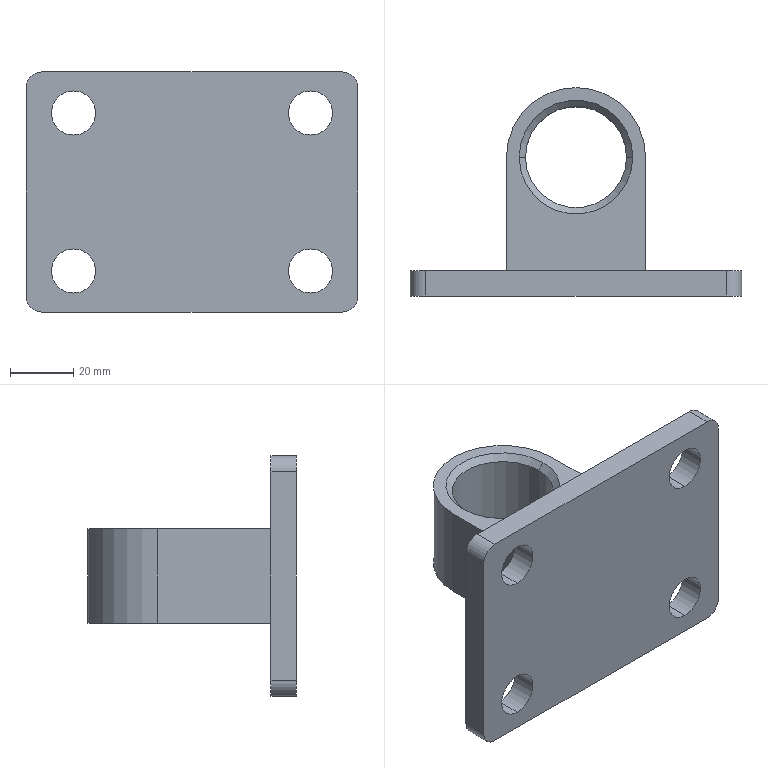Part | SolidWorks | features MirrorStock 1 | 2 solids | 30 faces | box 105 x 66 x 76 mm | volume 104524 mm3 | cylinder 15 | plane 11 | cone 4 | commonest cylinder face diameters 14 x8 10 x4 32 x2 44 x1
STEP:
#1=CARTESIAN_POINT('',(37.5,8.,18.));
#2=VERTEX_POINT('',#1);
#3=CARTESIAN_POINT('',(37.5,8.,32.));
#4=VERTEX_POINT('',#3);
#5=CARTESIAN_POINT('',(37.5,8.,25.));
#6=DIRECTION('',(0.,-1.,0.));
#7=DIRECTION('',(0.,0.,-1.));
#8=AXIS2_PLACEMENT_3D('',#5,#6,#7);
#9=CIRCLE('',#8,7.);
#10=EDGE_CURVE('',#2,#4,#9,.T.);
#11=ORIENTED_EDGE('',*,*,#10,.F.);
#12=CARTESIAN_POINT('',(37.5,0.,18.));
#13=VERTEX_POINT('',#12);
#14=CARTESIAN_POINT('',(37.5,8.,18.));
#15=DIRECTION('',(0.,-1.,0.));
#16=VECTOR('',#15,1000.);
#17=LINE('',#14,#16);
#18=EDGE_CURVE('',#2,#13,#17,.T.);
#19=ORIENTED_EDGE('',*,*,#18,.T.);
#20=CARTESIAN_POINT('',(37.5,0.,32.));
#21=VERTEX_POINT('',#20);
#22=CARTESIAN_POINT('',(37.5,0.,25.));
#23=DIRECTION('',(0.,-1.,0.));
#24=DIRECTION('',(0.,0.,-1.));
#25=AXIS2_PLACEMENT_3D('',#22,#23,#24);
#26=CIRCLE('',#25,7.);
#27=EDGE_CURVE('',#13,#21,#26,.T.);
#28=ORIENTED_EDGE('',*,*,#27,.T.);
#29=CARTESIAN_POINT('',(37.5,8.,32.));
#30=DIRECTION('',(0.,-1.,0.));
#31=VECTOR('',#30,1000.);
#32=LINE('',#29,#31);
#33=EDGE_CURVE('',#4,#21,#32,.T.);
#34=ORIENTED_EDGE('',*,*,#33,.F.);
#35=EDGE_LOOP('',(#11,#19,#28,#34));
#36=FACE_OUTER_BOUND('',#35,.T.);
#37=CARTESIAN_POINT('',(37.5,8.,25.));
#38=DIRECTION('',(0.,-1.,0.));
#39=DIRECTION('',(0.,0.,1.));
#40=AXIS2_PLACEMENT_3D('',#37,#38,#39);
#41=CYLINDRICAL_SURFACE('',#40,7.);
#42=ADVANCED_FACE('',(#36),#41,.F.);
#43=CARTESIAN_POINT('',(-37.5,8.,18.));
#44=VERTEX_POINT('',#43);
#45=CARTESIAN_POINT('',(-37.5,8.,32.));
#46=VERTEX_POINT('',#45);
#47=CARTESIAN_POINT('',(-37.5,8.,25.));
#48=DIRECTION('',(0.,-1.,0.));
#49=DIRECTION('',(0.,0.,1.));
#50=AXIS2_PLACEMENT_3D('',#47,#48,#49);
#51=CIRCLE('',#50,7.);
#52=EDGE_CURVE('',#44,#46,#51,.T.);
#53=ORIENTED_EDGE('',*,*,#52,.F.);
#54=CARTESIAN_POINT('',(-37.5,0.,18.));
#55=VERTEX_POINT('',#54);
#56=CARTESIAN_POINT('',(-37.5,8.,18.));
#57=DIRECTION('',(0.,-1.,0.));
#58=VECTOR('',#57,1000.);
#59=LINE('',#56,#58);
#60=EDGE_CURVE('',#44,#55,#59,.T.);
#61=ORIENTED_EDGE('',*,*,#60,.T.);
#62=CARTESIAN_POINT('',(-37.5,0.,32.));
#63=VERTEX_POINT('',#62);
#64=CARTESIAN_POINT('',(-37.5,0.,25.));
#65=DIRECTION('',(0.,-1.,0.));
#66=DIRECTION('',(0.,0.,1.));
#67=AXIS2_PLACEMENT_3D('',#64,#65,#66);
#68=CIRCLE('',#67,7.);
#69=EDGE_CURVE('',#55,#63,#68,.T.);
#70=ORIENTED_EDGE('',*,*,#69,.T.);
#71=CARTESIAN_POINT('',(-37.5,8.,32.));
#72=DIRECTION('',(0.,-1.,0.));
#73=VECTOR('',#72,1000.);
#74=LINE('',#71,#73);
#75=EDGE_CURVE('',#46,#63,#74,.T.);
#76=ORIENTED_EDGE('',*,*,#75,.F.);
#77=EDGE_LOOP('',(#53,#61,#70,#76));
#78=FACE_OUTER_BOUND('',#77,.T.);
#79=CARTESIAN_POINT('',(-37.5,8.,25.));
#80=DIRECTION('',(0.,-1.,0.));
#81=DIRECTION('',(0.,0.,1.));
#82=AXIS2_PLACEMENT_3D('',#79,#80,#81);
#83=CYLINDRICAL_SURFACE('',#82,7.);
#84=ADVANCED_FACE('',(#78),#83,.F.);
#85=CARTESIAN_POINT('',(37.5,8.,-32.));
#86=VERTEX_POINT('',#85);
#87=CARTESIAN_POINT('',(37.5,8.,-18.));
#88=VERTEX_POINT('',#87);
#89=CARTESIAN_POINT('',(37.5,8.,-25.));
#90=DIRECTION('',(0.,-1.,0.));
#91=DIRECTION('',(0.,0.,1.));
#92=AXIS2_PLACEMENT_3D('',#89,#90,#91);
#93=CIRCLE('',#92,7.);
#94=EDGE_CURVE('',#86,#88,#93,.T.);
#95=ORIENTED_EDGE('',*,*,#94,.F.);
#96=CARTESIAN_POINT('',(37.5,0.,-32.));
#97=VERTEX_POINT('',#96);
#98=CARTESIAN_POINT('',(37.5,8.,-32.));
#99=DIRECTION('',(0.,-1.,0.));
#100=VECTOR('',#99,1000.);
#101=LINE('',#98,#100);
#102=EDGE_CURVE('',#86,#97,#101,.T.);
#103=ORIENTED_EDGE('',*,*,#102,.T.);
#104=CARTESIAN_POINT('',(37.5,0.,-18.));
#105=VERTEX_POINT('',#104);
#106=CARTESIAN_POINT('',(37.5,0.,-25.));
#107=DIRECTION('',(0.,-1.,0.));
#108=DIRECTION('',(0.,0.,1.));
#109=AXIS2_PLACEMENT_3D('',#106,#107,#108);
#110=CIRCLE('',#109,7.);
#111=EDGE_CURVE('',#97,#105,#110,.T.);
#112=ORIENTED_EDGE('',*,*,#111,.T.);
#113=CARTESIAN_POINT('',(37.5,8.,-18.));
#114=DIRECTION('',(0.,-1.,0.));
#115=VECTOR('',#114,1000.);
#116=LINE('',#113,#115);
#117=EDGE_CURVE('',#88,#105,#116,.T.);
#118=ORIENTED_EDGE('',*,*,#117,.F.);
#119=EDGE_LOOP('',(#95,#103,#112,#118));
#120=FACE_OUTER_BOUND('',#119,.T.);
#121=CARTESIAN_POINT('',(37.5,8.,-25.));
#122=DIRECTION('',(0.,-1.,0.));
#123=DIRECTION('',(0.,0.,1.));
#124=AXIS2_PLACEMENT_3D('',#121,#122,#123);
#125=CYLINDRICAL_SURFACE('',#124,7.);
#126=ADVANCED_FACE('',(#120),#125,.F.);
#127=CARTESIAN_POINT('',(-37.5,8.,-32.));
#128=VERTEX_POINT('',#127);
#129=CARTESIAN_POINT('',(-37.5,8.,-18.));
#130=VERTEX_POINT('',#129);
#131=CARTESIAN_POINT('',(-37.5,8.,-25.));
#132=DIRECTION('',(0.,-1.,0.));
#133=DIRECTION('',(0.,0.,-1.));
#134=AXIS2_PLACEMENT_3D('',#131,#132,#133);
#135=CIRCLE('',#134,7.);
#136=EDGE_CURVE('',#128,#130,#135,.T.);
#137=ORIENTED_EDGE('',*,*,#136,.F.);
#138=CARTESIAN_POINT('',(-37.5,0.,-32.));
#139=VERTEX_POINT('',#138);
#140=CARTESIAN_POINT('',(-37.5,8.,-32.));
#141=DIRECTION('',(0.,-1.,0.));
#142=VECTOR('',#141,1000.);
#143=LINE('',#140,#142);
#144=EDGE_CURVE('',#128,#139,#143,.T.);
#145=ORIENTED_EDGE('',*,*,#144,.T.);
#146=CARTESIAN_POINT('',(-37.5,0.,-18.));
#147=VERTEX_POINT('',#146);
#148=CARTESIAN_POINT('',(-37.5,0.,-25.));
#149=DIRECTION('',(0.,-1.,0.));
#150=DIRECTION('',(0.,0.,-1.));
#151=AXIS2_PLACEMENT_3D('',#148,#149,#150);
#152=CIRCLE('',#151,7.);
#153=EDGE_CURVE('',#139,#147,#152,.T.);
#154=ORIENTED_EDGE('',*,*,#153,.T.);
#155=CARTESIAN_POINT('',(-37.5,8.,-18.));
#156=DIRECTION('',(0.,-1.,0.));
#157=VECTOR('',#156,1000.);
#158=LINE('',#155,#157);
#159=EDGE_CURVE('',#130,#147,#158,.T.);
#160=ORIENTED_EDGE('',*,*,#159,.F.);
#161=EDGE_LOOP('',(#137,#145,#154,#160));
#162=FACE_OUTER_BOUND('',#161,.T.);
#163=CARTESIAN_POINT('',(-37.5,8.,-25.));
#164=DIRECTION('',(0.,-1.,0.));
#165=DIRECTION('',(0.,0.,1.));
#166=AXIS2_PLACEMENT_3D('',#163,#164,#165);
#167=CYLINDRICAL_SURFACE('',#166,7.);
#168=ADVANCED_FACE('',(#162),#167,.F.);
#169=CARTESIAN_POINT('',(-37.5,8.,25.));
#170=DIRECTION('',(0.,-1.,0.));
#171=DIRECTION('',(0.,0.,1.));
#172=AXIS2_PLACEMENT_3D('',#169,#170,#171);
#173=CIRCLE('',#172,7.);
#174=EDGE_CURVE('',#46,#44,#173,.T.);
#175=ORIENTED_EDGE('',*,*,#174,.T.);
#176=ORIENTED_EDGE('',*,*,#52,.T.);
#177=EDGE_LOOP('',(#175,#176));
#178=FACE_BOUND('',#177,.T.);
#179=CARTESIAN_POINT('',(-37.5,8.,-25.));
#180=DIRECTION('',(0.,-1.,0.));
#181=DIRECTION('',(0.,0.,-1.));
#182=AXIS2_PLACEMENT_3D('',#179,#180,#181);
#183=CIRCLE('',#182,7.);
#184=EDGE_CURVE('',#130,#128,#183,.T.);
#185=ORIENTED_EDGE('',*,*,#184,.T.);
#186=ORIENTED_EDGE('',*,*,#136,.T.);
#187=EDGE_LOOP('',(#185,#186));
#188=FACE_BOUND('',#187,.T.);
#189=CARTESIAN_POINT('',(47.5,8.,-38.));
#190=VERTEX_POINT('',#189);
#191=CARTESIAN_POINT('',(52.5,8.,-33.));
#192=VERTEX_POINT('',#191);
#193=CARTESIAN_POINT('',(47.5,8.,-33.));
#194=DIRECTION('',(0.,-1.,0.));
#195=DIRECTION('',(0.,0.,-1.));
#196=AXIS2_PLACEMENT_3D('',#193,#194,#195);
#197=CIRCLE('',#196,5.);
#198=EDGE_CURVE('',#190,#192,#197,.T.);
#199=ORIENTED_EDGE('',*,*,#198,.F.);
#200=CARTESIAN_POINT('',(-47.5,8.,-38.));
#201=VERTEX_POINT('',#200);
#202=CARTESIAN_POINT('',(-47.5,8.,-38.));
#203=DIRECTION('',(1.,0.,0.));
#204=VECTOR('',#203,1000.);
#205=LINE('',#202,#204);
#206=EDGE_CURVE('',#201,#190,#205,.T.);
#207=ORIENTED_EDGE('',*,*,#206,.F.);
#208=CARTESIAN_POINT('',(-52.5,8.,-33.));
#209=VERTEX_POINT('',#208);
#210=CARTESIAN_POINT('',(-47.5,8.,-33.));
#211=DIRECTION('',(0.,-1.,0.));
#212=DIRECTION('',(0.,0.,1.));
#213=AXIS2_PLACEMENT_3D('',#210,#211,#212);
#214=CIRCLE('',#213,5.);
#215=EDGE_CURVE('',#209,#201,#214,.T.);
#216=ORIENTED_EDGE('',*,*,#215,.F.);
#217=CARTESIAN_POINT('',(-52.5,8.,33.));
#218=VERTEX_POINT('',#217);
#219=CARTESIAN_POINT('',(-52.5,8.,-33.));
#220=DIRECTION('',(0.,0.,-1.));
#221=VECTOR('',#220,1000.);
#222=LINE('',#219,#221);
#223=EDGE_CURVE('',#218,#209,#222,.T.);
#224=ORIENTED_EDGE('',*,*,#223,.F.);
#225=CARTESIAN_POINT('',(-47.5,8.,38.));
#226=VERTEX_POINT('',#225);
#227=CARTESIAN_POINT('',(-47.5,8.,33.));
#228=DIRECTION('',(0.,-1.,0.));
#229=DIRECTION('',(0.,0.,1.));
#230=AXIS2_PLACEMENT_3D('',#227,#228,#229);
#231=CIRCLE('',#230,5.);
#232=EDGE_CURVE('',#226,#218,#231,.T.);
#233=ORIENTED_EDGE('',*,*,#232,.F.);
#234=CARTESIAN_POINT('',(47.5,8.,38.));
#235=VERTEX_POINT('',#234);
#236=CARTESIAN_POINT('',(-47.5,8.,38.));
#237=DIRECTION('',(-1.,0.,0.));
#238=VECTOR('',#237,1000.);
#239=LINE('',#236,#238);
#240=EDGE_CURVE('',#235,#226,#239,.T.);
#241=ORIENTED_EDGE('',*,*,#240,.F.);
#242=CARTESIAN_POINT('',(52.5,8.,33.));
#243=VERTEX_POINT('',#242);
#244=CARTESIAN_POINT('',(47.5,8.,33.));
#245=DIRECTION('',(0.,-1.,0.));
#246=DIRECTION('',(0.,0.,1.));
#247=AXIS2_PLACEMENT_3D('',#244,#245,#246);
#248=CIRCLE('',#247,5.);
#249=EDGE_CURVE('',#243,#235,#248,.T.);
#250=ORIENTED_EDGE('',*,*,#249,.F.);
#251=CARTESIAN_POINT('',(52.5,8.,-33.));
#252=DIRECTION('',(0.,0.,1.));
#253=VECTOR('',#252,1000.);
#254=LINE('',#251,#253);
#255=EDGE_CURVE('',#192,#243,#254,.T.);
#256=ORIENTED_EDGE('',*,*,#255,.F.);
#257=EDGE_LOOP('',(#199,#207,#216,#224,#233,#241,#250,#256));
#258=FACE_OUTER_BOUND('',#257,.T.);
#259=CARTESIAN_POINT('',(37.5,8.,-25.));
#260=DIRECTION('',(0.,-1.,0.));
#261=DIRECTION('',(0.,0.,1.));
#262=AXIS2_PLACEMENT_3D('',#259,#260,#261);
#263=CIRCLE('',#262,7.);
#264=EDGE_CURVE('',#88,#86,#263,.T.);
#265=ORIENTED_EDGE('',*,*,#264,.T.);
#266=ORIENTED_EDGE('',*,*,#94,.T.);
#267=EDGE_LOOP('',(#265,#266));
#268=FACE_BOUND('',#267,.T.);
#269=CARTESIAN_POINT('',(37.5,8.,25.));
#270=DIRECTION('',(0.,-1.,0.));
#271=DIRECTION('',(0.,0.,-1.));
#272=AXIS2_PLACEMENT_3D('',#269,#270,#271);
#273=CIRCLE('',#272,7.);
#274=EDGE_CURVE('',#4,#2,#273,.T.);
#275=ORIENTED_EDGE('',*,*,#274,.T.);
#276=ORIENTED_EDGE('',*,*,#10,.T.);
#277=EDGE_LOOP('',(#275,#276));
#278=FACE_BOUND('',#277,.T.);
#279=CARTESIAN_POINT('',(47.5,8.,-33.));
#280=DIRECTION('',(0.,1.,0.));
#281=DIRECTION('',(0.,0.,-1.));
#282=AXIS2_PLACEMENT_3D('',#279,#280,#281);
#283=PLANE('',#282);
#284=ADVANCED_FACE('',(#178,#188,#258,#268,#278),#283,.T.);
#285=CARTESIAN_POINT('',(47.5,0.,-38.));
#286=VERTEX_POINT('',#285);
#287=CARTESIAN_POINT('',(52.5,0.,-33.));
#288=VERTEX_POINT('',#287);
#289=CARTESIAN_POINT('',(47.5,0.,-33.));
#290=DIRECTION('',(0.,-1.,0.));
#291=DIRECTION('',(0.,0.,-1.));
#292=AXIS2_PLACEMENT_3D('',#289,#290,#291);
#293=CIRCLE('',#292,5.);
#294=EDGE_CURVE('',#286,#288,#293,.T.);
#295=ORIENTED_EDGE('',*,*,#294,.T.);
#296=CARTESIAN_POINT('',(52.5,0.,33.));
#297=VERTEX_POINT('',#296);
#298=CARTESIAN_POINT('',(52.5,0.,-33.));
#299=DIRECTION('',(0.,0.,1.));
#300=VECTOR('',#299,1000.);
#301=LINE('',#298,#300);
#302=EDGE_CURVE('',#288,#297,#301,.T.);
#303=ORIENTED_EDGE('',*,*,#302,.T.);
#304=CARTESIAN_POINT('',(47.5,0.,38.));
#305=VERTEX_POINT('',#304);
#306=CARTESIAN_POINT('',(47.5,0.,33.));
#307=DIRECTION('',(0.,-1.,0.));
#308=DIRECTION('',(0.,0.,1.));
#309=AXIS2_PLACEMENT_3D('',#306,#307,#308);
#310=CIRCLE('',#309,5.);
#311=EDGE_CURVE('',#297,#305,#310,.T.);
#312=ORIENTED_EDGE('',*,*,#311,.T.);
#313=CARTESIAN_POINT('',(-47.5,0.,38.));
#314=VERTEX_POINT('',#313);
#315=CARTESIAN_POINT('',(-47.5,0.,38.));
#316=DIRECTION('',(-1.,0.,0.));
#317=VECTOR('',#316,1000.);
#318=LINE('',#315,#317);
#319=EDGE_CURVE('',#305,#314,#318,.T.);
#320=ORIENTED_EDGE('',*,*,#319,.T.);
#321=CARTESIAN_POINT('',(-52.5,0.,33.));
#322=VERTEX_POINT('',#321);
#323=CARTESIAN_POINT('',(-47.5,0.,33.));
#324=DIRECTION('',(0.,-1.,0.));
#325=DIRECTION('',(0.,0.,1.));
#326=AXIS2_PLACEMENT_3D('',#323,#324,#325);
#327=CIRCLE('',#326,5.);
#328=EDGE_CURVE('',#314,#322,#327,.T.);
#329=ORIENTED_EDGE('',*,*,#328,.T.);
#330=CARTESIAN_POINT('',(-52.5,0.,-33.));
#331=VERTEX_POINT('',#330);
#332=CARTESIAN_POINT('',(-52.5,0.,-33.));
#333=DIRECTION('',(0.,0.,-1.));
#334=VECTOR('',#333,1000.);
#335=LINE('',#332,#334);
#336=EDGE_CURVE('',#322,#331,#335,.T.);
#337=ORIENTED_EDGE('',*,*,#336,.T.);
#338=CARTESIAN_POINT('',(-47.5,0.,-38.));
#339=VERTEX_POINT('',#338);
#340=CARTESIAN_POINT('',(-47.5,0.,-33.));
#341=DIRECTION('',(0.,-1.,0.));
#342=DIRECTION('',(0.,0.,1.));
#343=AXIS2_PLACEMENT_3D('',#340,#341,#342);
#344=CIRCLE('',#343,5.);
#345=EDGE_CURVE('',#331,#339,#344,.T.);
#346=ORIENTED_EDGE('',*,*,#345,.T.);
#347=CARTESIAN_POINT('',(-47.5,0.,-38.));
#348=DIRECTION('',(1.,0.,0.));
#349=VECTOR('',#348,1000.);
#350=LINE('',#347,#349);
#351=EDGE_CURVE('',#339,#286,#350,.T.);
#352=ORIENTED_EDGE('',*,*,#351,.T.);
#353=EDGE_LOOP('',(#295,#303,#312,#320,#329,#337,#346,#352));
#354=FACE_OUTER_BOUND('',#353,.T.);
#355=CARTESIAN_POINT('',(-37.5,0.,-25.));
#356=DIRECTION('',(0.,-1.,0.));
#357=DIRECTION('',(0.,0.,-1.));
#358=AXIS2_PLACEMENT_3D('',#355,#356,#357);
#359=CIRCLE('',#358,7.);
#360=EDGE_CURVE('',#147,#139,#359,.T.);
#361=ORIENTED_EDGE('',*,*,#360,.F.);
#362=ORIENTED_EDGE('',*,*,#153,.F.);
#363=EDGE_LOOP('',(#361,#362));
#364=FACE_BOUND('',#363,.T.);
#365=CARTESIAN_POINT('',(37.5,0.,-25.));
#366=DIRECTION('',(0.,-1.,0.));
#367=DIRECTION('',(0.,0.,1.));
#368=AXIS2_PLACEMENT_3D('',#365,#366,#367);
#369=CIRCLE('',#368,7.);
#370=EDGE_CURVE('',#105,#97,#369,.T.);
#371=ORIENTED_EDGE('',*,*,#370,.F.);
#372=ORIENTED_EDGE('',*,*,#111,.F.);
#373=EDGE_LOOP('',(#371,#372));
#374=FACE_BOUND('',#373,.T.);
#375=CARTESIAN_POINT('',(-37.5,0.,25.));
#376=DIRECTION('',(0.,-1.,0.));
#377=DIRECTION('',(0.,0.,1.));
#378=AXIS2_PLACEMENT_3D('',#375,#376,#377);
#379=CIRCLE('',#378,7.);
#380=EDGE_CURVE('',#63,#55,#379,.T.);
#381=ORIENTED_EDGE('',*,*,#380,.F.);
#382=ORIENTED_EDGE('',*,*,#69,.F.);
#383=EDGE_LOOP('',(#381,#382));
#384=FACE_BOUND('',#383,.T.);
#385=CARTESIAN_POINT('',(37.5,0.,25.));
#386=DIRECTION('',(0.,-1.,0.));
#387=DIRECTION('',(0.,0.,-1.));
#388=AXIS2_PLACEMENT_3D('',#385,#386,#387);
#389=CIRCLE('',#388,7.);
#390=EDGE_CURVE('',#21,#13,#389,.T.);
#391=ORIENTED_EDGE('',*,*,#390,.F.);
#392=ORIENTED_EDGE('',*,*,#27,.F.);
#393=EDGE_LOOP('',(#391,#392));
#394=FACE_BOUND('',#393,.T.);
#395=CARTESIAN_POINT('',(47.5,0.,-33.));
#396=DIRECTION('',(0.,1.,0.));
#397=DIRECTION('',(0.,0.,-1.));
#398=AXIS2_PLACEMENT_3D('',#395,#396,#397);
#399=PLANE('',#398);
#400=ADVANCED_FACE('',(#354,#364,#374,#384,#394),#399,.F.);
#401=ORIENTED_EDGE('',*,*,#294,.F.);
#402=CARTESIAN_POINT('',(47.5,8.,-38.));
#403=DIRECTION('',(0.,-1.,0.));
#404=VECTOR('',#403,1000.);
#405=LINE('',#402,#404);
#406=EDGE_CURVE('',#190,#286,#405,.T.);
#407=ORIENTED_EDGE('',*,*,#406,.F.);
#408=ORIENTED_EDGE('',*,*,#198,.T.);
#409=CARTESIAN_POINT('',(52.5,8.,-33.));
#410=DIRECTION('',(0.,-1.,0.));
#411=VECTOR('',#410,1000.);
#412=LINE('',#409,#411);
#413=EDGE_CURVE('',#192,#288,#412,.T.);
#414=ORIENTED_EDGE('',*,*,#413,.T.);
#415=EDGE_LOOP('',(#401,#407,#408,#414));
#416=FACE_OUTER_BOUND('',#415,.T.);
#417=CARTESIAN_POINT('',(47.5,8.,-33.));
#418=DIRECTION('',(0.,-1.,0.));
#419=DIRECTION('',(0.,0.,1.));
#420=AXIS2_PLACEMENT_3D('',#417,#418,#419);
#421=CYLINDRICAL_SURFACE('',#420,5.);
#422=ADVANCED_FACE('',(#416),#421,.T.);
#423=ORIENTED_EDGE('',*,*,#302,.F.);
#424=ORIENTED_EDGE('',*,*,#413,.F.);
#425=ORIENTED_EDGE('',*,*,#255,.T.);
#426=CARTESIAN_POINT('',(52.5,8.,33.));
#427=DIRECTION('',(0.,-1.,0.));
#428=VECTOR('',#427,1000.);
#429=LINE('',#426,#428);
#430=EDGE_CURVE('',#243,#297,#429,.T.);
#431=ORIENTED_EDGE('',*,*,#430,.T.);
#432=EDGE_LOOP('',(#423,#424,#425,#431));
#433=FACE_OUTER_BOUND('',#432,.T.);
#434=CARTESIAN_POINT('',(52.5,8.,-33.));
#435=DIRECTION('',(-1.,0.,0.));
#436=DIRECTION('',(0.,0.,-1.));
#437=AXIS2_PLACEMENT_3D('',#434,#435,#436);
#438=PLANE('',#437);
#439=ADVANCED_FACE('',(#433),#438,.F.);
#440=ORIENTED_EDGE('',*,*,#311,.F.);
#441=ORIENTED_EDGE('',*,*,#430,.F.);
#442=ORIENTED_EDGE('',*,*,#249,.T.);
#443=CARTESIAN_POINT('',(47.5,8.,38.));
#444=DIRECTION('',(0.,-1.,0.));
#445=VECTOR('',#444,1000.);
#446=LINE('',#443,#445);
#447=EDGE_CURVE('',#235,#305,#446,.T.);
#448=ORIENTED_EDGE('',*,*,#447,.T.);
#449=EDGE_LOOP('',(#440,#441,#442,#448));
#450=FACE_OUTER_BOUND('',#449,.T.);
#451=CARTESIAN_POINT('',(47.5,8.,33.));
#452=DIRECTION('',(0.,-1.,0.));
#453=DIRECTION('',(0.,0.,1.));
#454=AXIS2_PLACEMENT_3D('',#451,#452,#453);
#455=CYLINDRICAL_SURFACE('',#454,5.);
#456=ADVANCED_FACE('',(#450),#455,.T.);
#457=ORIENTED_EDGE('',*,*,#319,.F.);
#458=ORIENTED_EDGE('',*,*,#447,.F.);
#459=ORIENTED_EDGE('',*,*,#240,.T.);
#460=CARTESIAN_POINT('',(-47.5,8.,38.));
#461=DIRECTION('',(0.,-1.,0.));
#462=VECTOR('',#461,1000.);
#463=LINE('',#460,#462);
#464=EDGE_CURVE('',#226,#314,#463,.T.);
#465=ORIENTED_EDGE('',*,*,#464,.T.);
#466=EDGE_LOOP('',(#457,#458,#459,#465));
#467=FACE_OUTER_BOUND('',#466,.T.);
#468=CARTESIAN_POINT('',(-47.5,8.,38.));
#469=DIRECTION('',(0.,0.,-1.));
#470=DIRECTION('',(1.,0.,0.));
#471=AXIS2_PLACEMENT_3D('',#468,#469,#470);
#472=PLANE('',#471);
#473=ADVANCED_FACE('',(#467),#472,.F.);
#474=ORIENTED_EDGE('',*,*,#328,.F.);
#475=ORIENTED_EDGE('',*,*,#464,.F.);
#476=ORIENTED_EDGE('',*,*,#232,.T.);
#477=CARTESIAN_POINT('',(-52.5,8.,33.));
#478=DIRECTION('',(0.,-1.,0.));
#479=VECTOR('',#478,1000.);
#480=LINE('',#477,#479);
#481=EDGE_CURVE('',#218,#322,#480,.T.);
#482=ORIENTED_EDGE('',*,*,#481,.T.);
#483=EDGE_LOOP('',(#474,#475,#476,#482));
#484=FACE_OUTER_BOUND('',#483,.T.);
#485=CARTESIAN_POINT('',(-47.5,8.,33.));
#486=DIRECTION('',(0.,-1.,0.));
#487=DIRECTION('',(0.,0.,1.));
#488=AXIS2_PLACEMENT_3D('',#485,#486,#487);
#489=CYLINDRICAL_SURFACE('',#488,5.);
#490=ADVANCED_FACE('',(#484),#489,.T.);
#491=ORIENTED_EDGE('',*,*,#336,.F.);
#492=ORIENTED_EDGE('',*,*,#481,.F.);
#493=ORIENTED_EDGE('',*,*,#223,.T.);
#494=CARTESIAN_POINT('',(-52.5,8.,-33.));
#495=DIRECTION('',(0.,-1.,0.));
#496=VECTOR('',#495,1000.);
#497=LINE('',#494,#496);
#498=EDGE_CURVE('',#209,#331,#497,.T.);
#499=ORIENTED_EDGE('',*,*,#498,.T.);
#500=EDGE_LOOP('',(#491,#492,#493,#499));
#501=FACE_OUTER_BOUND('',#500,.T.);
#502=CARTESIAN_POINT('',(-52.5,8.,-33.));
#503=DIRECTION('',(1.,0.,0.));
#504=DIRECTION('',(0.,0.,1.));
#505=AXIS2_PLACEMENT_3D('',#502,#503,#504);
#506=PLANE('',#505);
#507=ADVANCED_FACE('',(#501),#506,.F.);
#508=ORIENTED_EDGE('',*,*,#345,.F.);
#509=ORIENTED_EDGE('',*,*,#498,.F.);
#510=ORIENTED_EDGE('',*,*,#215,.T.);
#511=CARTESIAN_POINT('',(-47.5,8.,-38.));
#512=DIRECTION('',(0.,-1.,0.));
#513=VECTOR('',#512,1000.);
#514=LINE('',#511,#513);
#515=EDGE_CURVE('',#201,#339,#514,.T.);
#516=ORIENTED_EDGE('',*,*,#515,.T.);
#517=EDGE_LOOP('',(#508,#509,#510,#516));
#518=FACE_OUTER_BOUND('',#517,.T.);
#519=CARTESIAN_POINT('',(-47.5,8.,-33.));
#520=DIRECTION('',(0.,-1.,0.));
#521=DIRECTION('',(0.,0.,1.));
#522=AXIS2_PLACEMENT_3D('',#519,#520,#521);
#523=CYLINDRICAL_SURFACE('',#522,5.);
#524=ADVANCED_FACE('',(#518),#523,.T.);
#525=ORIENTED_EDGE('',*,*,#351,.F.);
#526=ORIENTED_EDGE('',*,*,#515,.F.);
#527=ORIENTED_EDGE('',*,*,#206,.T.);
#528=ORIENTED_EDGE('',*,*,#406,.T.);
#529=EDGE_LOOP('',(#525,#526,#527,#528));
#530=FACE_OUTER_BOUND('',#529,.T.);
#531=CARTESIAN_POINT('',(-47.5,8.,-38.));
#532=DIRECTION('',(0.,0.,1.));
#533=DIRECTION('',(-1.,0.,0.));
#534=AXIS2_PLACEMENT_3D('',#531,#532,#533);
#535=PLANE('',#534);
#536=ADVANCED_FACE('',(#530),#535,.F.);
#537=ORIENTED_EDGE('',*,*,#144,.F.);
#538=ORIENTED_EDGE('',*,*,#184,.F.);
#539=ORIENTED_EDGE('',*,*,#159,.T.);
#540=ORIENTED_EDGE('',*,*,#360,.T.);
#541=EDGE_LOOP('',(#537,#538,#539,#540));
#542=FACE_OUTER_BOUND('',#541,.T.);
#543=CARTESIAN_POINT('',(-37.5,8.,-25.));
#544=DIRECTION('',(0.,-1.,0.));
#545=DIRECTION('',(0.,0.,1.));
#546=AXIS2_PLACEMENT_3D('',#543,#544,#545);
#547=CYLINDRICAL_SURFACE('',#546,7.);
#548=ADVANCED_FACE('',(#542),#547,.F.);
#549=ORIENTED_EDGE('',*,*,#102,.F.);
#550=ORIENTED_EDGE('',*,*,#264,.F.);
#551=ORIENTED_EDGE('',*,*,#117,.T.);
#552=ORIENTED_EDGE('',*,*,#370,.T.);
#553=EDGE_LOOP('',(#549,#550,#551,#552));
#554=FACE_OUTER_BOUND('',#553,.T.);
#555=CARTESIAN_POINT('',(37.5,8.,-25.));
#556=DIRECTION('',(0.,-1.,0.));
#557=DIRECTION('',(0.,0.,1.));
#558=AXIS2_PLACEMENT_3D('',#555,#556,#557);
#559=CYLINDRICAL_SURFACE('',#558,7.);
#560=ADVANCED_FACE('',(#554),#559,.F.);
#561=ORIENTED_EDGE('',*,*,#60,.F.);
#562=ORIENTED_EDGE('',*,*,#174,.F.);
#563=ORIENTED_EDGE('',*,*,#75,.T.);
#564=ORIENTED_EDGE('',*,*,#380,.T.);
#565=EDGE_LOOP('',(#561,#562,#563,#564));
#566=FACE_OUTER_BOUND('',#565,.T.);
#567=CARTESIAN_POINT('',(-37.5,8.,25.));
#568=DIRECTION('',(0.,-1.,0.));
#569=DIRECTION('',(0.,0.,1.));
#570=AXIS2_PLACEMENT_3D('',#567,#568,#569);
#571=CYLINDRICAL_SURFACE('',#570,7.);
#572=ADVANCED_FACE('',(#566),#571,.F.);
#573=ORIENTED_EDGE('',*,*,#18,.F.);
#574=ORIENTED_EDGE('',*,*,#274,.F.);
#575=ORIENTED_EDGE('',*,*,#33,.T.);
#576=ORIENTED_EDGE('',*,*,#390,.T.);
#577=EDGE_LOOP('',(#573,#574,#575,#576));
#578=FACE_OUTER_BOUND('',#577,.T.);
#579=CARTESIAN_POINT('',(37.5,8.,25.));
#580=DIRECTION('',(0.,-1.,0.));
#581=DIRECTION('',(0.,0.,1.));
#582=AXIS2_PLACEMENT_3D('',#579,#580,#581);
#583=CYLINDRICAL_SURFACE('',#582,7.);
#584=ADVANCED_FACE('',(#578),#583,.F.);
#585=CLOSED_SHELL('',(#42,#84,#126,#168,#284,#400,#422,#439,#456,#473,#490,#507,#524,#536,#548,#560,#572,#584));
#586=MANIFOLD_SOLID_BREP('',#585);
#587=CARTESIAN_POINT('',(-16.,44.,13.));
#588=VERTEX_POINT('',#587);
#589=CARTESIAN_POINT('',(16.,44.,13.));
#590=VERTEX_POINT('',#589);
#591=CARTESIAN_POINT('',(0.,44.,13.));
#592=DIRECTION('',(0.,0.,-1.));
#593=DIRECTION('',(1.,0.,0.));
#594=AXIS2_PLACEMENT_3D('',#591,#592,#593);
#595=CIRCLE('',#594,16.);
#596=EDGE_CURVE('',#588,#590,#595,.T.);
#597=ORIENTED_EDGE('',*,*,#596,.T.);
#598=CARTESIAN_POINT('',(18.,44.,15.));
#599=VERTEX_POINT('',#598);
#600=CARTESIAN_POINT('',(18.,44.,15.));
#601=DIRECTION('',(0.7071,0.,0.7071));
#602=VECTOR('',#601,1000.);
#603=LINE('',#600,#602);
#604=EDGE_CURVE('',#590,#599,#603,.T.);
#605=ORIENTED_EDGE('',*,*,#604,.T.);
#606=CARTESIAN_POINT('',(-18.,44.,15.));
#607=VERTEX_POINT('',#606);
#608=CARTESIAN_POINT('',(0.,44.,15.));
#609=DIRECTION('',(0.,0.,1.));
#610=DIRECTION('',(1.,0.,0.));
#611=AXIS2_PLACEMENT_3D('',#608,#609,#610);
#612=CIRCLE('',#611,18.);
#613=EDGE_CURVE('',#599,#607,#612,.T.);
#614=ORIENTED_EDGE('',*,*,#613,.T.);
#615=CARTESIAN_POINT('',(-18.,44.,15.));
#616=DIRECTION('',(-0.7071,0.,0.7071));
#617=VECTOR('',#616,1000.);
#618=LINE('',#615,#617);
#619=EDGE_CURVE('',#588,#607,#618,.T.);
#620=ORIENTED_EDGE('',*,*,#619,.F.);
#621=EDGE_LOOP('',(#597,#605,#614,#620));
#622=FACE_OUTER_BOUND('',#621,.T.);
#623=CARTESIAN_POINT('',(0.,44.,15.));
#624=DIRECTION('',(0.,0.,1.));
#625=DIRECTION('',(-1.,0.,0.));
#626=AXIS2_PLACEMENT_3D('',#623,#624,#625);
#627=CONICAL_SURFACE('',#626,18.,0.7854);
#628=ADVANCED_FACE('',(#622),#627,.F.);
#629=CARTESIAN_POINT('',(16.,44.,-13.));
#630=VERTEX_POINT('',#629);
#631=CARTESIAN_POINT('',(-16.,44.,-13.));
#632=VERTEX_POINT('',#631);
#633=CARTESIAN_POINT('',(0.,44.,-13.));
#634=DIRECTION('',(0.,0.,1.));
#635=DIRECTION('',(1.,0.,0.));
#636=AXIS2_PLACEMENT_3D('',#633,#634,#635);
#637=CIRCLE('',#636,16.);
#638=EDGE_CURVE('',#630,#632,#637,.T.);
#639=ORIENTED_EDGE('',*,*,#638,.T.);
#640=CARTESIAN_POINT('',(-18.,44.,-15.));
#641=VERTEX_POINT('',#640);
#642=CARTESIAN_POINT('',(-16.,44.,-13.));
#643=DIRECTION('',(-0.7071,0.,-0.7071));
#644=VECTOR('',#643,1000.);
#645=LINE('',#642,#644);
#646=EDGE_CURVE('',#632,#641,#645,.T.);
#647=ORIENTED_EDGE('',*,*,#646,.T.);
#648=CARTESIAN_POINT('',(18.,44.,-15.));
#649=VERTEX_POINT('',#648);
#650=CARTESIAN_POINT('',(0.,44.,-15.));
#651=DIRECTION('',(0.,0.,-1.));
#652=DIRECTION('',(1.,0.,0.));
#653=AXIS2_PLACEMENT_3D('',#650,#651,#652);
#654=CIRCLE('',#653,18.);
#655=EDGE_CURVE('',#641,#649,#654,.T.);
#656=ORIENTED_EDGE('',*,*,#655,.T.);
#657=CARTESIAN_POINT('',(16.,44.,-13.));
#658=DIRECTION('',(0.7071,0.,-0.7071));
#659=VECTOR('',#658,1000.);
#660=LINE('',#657,#659);
#661=EDGE_CURVE('',#630,#649,#660,.T.);
#662=ORIENTED_EDGE('',*,*,#661,.F.);
#663=EDGE_LOOP('',(#639,#647,#656,#662));
#664=FACE_OUTER_BOUND('',#663,.T.);
#665=CARTESIAN_POINT('',(0.,44.,-13.));
#666=DIRECTION('',(0.,0.,-1.));
#667=DIRECTION('',(1.,0.,0.));
#668=AXIS2_PLACEMENT_3D('',#665,#666,#667);
#669=CONICAL_SURFACE('',#668,16.,0.7854);
#670=ADVANCED_FACE('',(#664),#669,.F.);
#671=ORIENTED_EDGE('',*,*,#596,.F.);
#672=CARTESIAN_POINT('',(-16.,44.,15.));
#673=DIRECTION('',(0.,0.,-1.));
#674=VECTOR('',#673,1000.);
#675=LINE('',#672,#674);
#676=EDGE_CURVE('',#588,#632,#675,.T.);
#677=ORIENTED_EDGE('',*,*,#676,.T.);
#678=ORIENTED_EDGE('',*,*,#638,.F.);
#679=CARTESIAN_POINT('',(16.,44.,15.));
#680=DIRECTION('',(0.,0.,-1.));
#681=VECTOR('',#680,1000.);
#682=LINE('',#679,#681);
#683=EDGE_CURVE('',#590,#630,#682,.T.);
#684=ORIENTED_EDGE('',*,*,#683,.F.);
#685=EDGE_LOOP('',(#671,#677,#678,#684));
#686=FACE_OUTER_BOUND('',#685,.T.);
#687=CARTESIAN_POINT('',(0.,44.,15.));
#688=DIRECTION('',(0.,0.,-1.));
#689=DIRECTION('',(1.,0.,0.));
#690=AXIS2_PLACEMENT_3D('',#687,#688,#689);
#691=CYLINDRICAL_SURFACE('',#690,16.);
#692=ADVANCED_FACE('',(#686),#691,.F.);
#693=CARTESIAN_POINT('',(22.,8.,-15.));
#694=VERTEX_POINT('',#693);
#695=CARTESIAN_POINT('',(22.,44.,-15.));
#696=VERTEX_POINT('',#695);
#697=CARTESIAN_POINT('',(22.,44.,-15.));
#698=DIRECTION('',(0.,1.,0.));
#699=VECTOR('',#698,1000.);
#700=LINE('',#697,#699);
#701=EDGE_CURVE('',#694,#696,#700,.T.);
#702=ORIENTED_EDGE('',*,*,#701,.T.);
#703=CARTESIAN_POINT('',(22.,44.,15.));
#704=VERTEX_POINT('',#703);
#705=CARTESIAN_POINT('',(22.,44.,15.));
#706=DIRECTION('',(0.,0.,-1.));
#707=VECTOR('',#706,1000.);
#708=LINE('',#705,#707);
#709=EDGE_CURVE('',#704,#696,#708,.T.);
#710=ORIENTED_EDGE('',*,*,#709,.F.);
#711=CARTESIAN_POINT('',(22.,8.,15.));
#712=VERTEX_POINT('',#711);
#713=CARTESIAN_POINT('',(22.,44.,15.));
#714=DIRECTION('',(0.,1.,0.));
#715=VECTOR('',#714,1000.);
#716=LINE('',#713,#715);
#717=EDGE_CURVE('',#712,#704,#716,.T.);
#718=ORIENTED_EDGE('',*,*,#717,.F.);
#719=CARTESIAN_POINT('',(22.,8.,15.));
#720=DIRECTION('',(0.,0.,-1.));
#721=VECTOR('',#720,1000.);
#722=LINE('',#719,#721);
#723=EDGE_CURVE('',#712,#694,#722,.T.);
#724=ORIENTED_EDGE('',*,*,#723,.T.);
#725=EDGE_LOOP('',(#702,#710,#718,#724));
#726=FACE_OUTER_BOUND('',#725,.T.);
#727=CARTESIAN_POINT('',(22.,44.,15.));
#728=DIRECTION('',(1.,0.,0.));
#729=DIRECTION('',(0.,1.,0.));
#730=AXIS2_PLACEMENT_3D('',#727,#728,#729);
#731=PLANE('',#730);
#732=ADVANCED_FACE('',(#726),#731,.T.);
#733=CARTESIAN_POINT('',(-22.,8.,-15.));
#734=VERTEX_POINT('',#733);
#735=CARTESIAN_POINT('',(-22.,8.,-15.));
#736=DIRECTION('',(1.,0.,0.));
#737=VECTOR('',#736,1000.);
#738=LINE('',#735,#737);
#739=EDGE_CURVE('',#734,#694,#738,.T.);
#740=ORIENTED_EDGE('',*,*,#739,.T.);
#741=ORIENTED_EDGE('',*,*,#723,.F.);
#742=CARTESIAN_POINT('',(-22.,8.,15.));
#743=VERTEX_POINT('',#742);
#744=CARTESIAN_POINT('',(-22.,8.,15.));
#745=DIRECTION('',(1.,0.,0.));
#746=VECTOR('',#745,1000.);
#747=LINE('',#744,#746);
#748=EDGE_CURVE('',#743,#712,#747,.T.);
#749=ORIENTED_EDGE('',*,*,#748,.F.);
#750=CARTESIAN_POINT('',(-22.,8.,15.));
#751=DIRECTION('',(0.,0.,-1.));
#752=VECTOR('',#751,1000.);
#753=LINE('',#750,#752);
#754=EDGE_CURVE('',#743,#734,#753,.T.);
#755=ORIENTED_EDGE('',*,*,#754,.T.);
#756=EDGE_LOOP('',(#740,#741,#749,#755));
#757=FACE_OUTER_BOUND('',#756,.T.);
#758=CARTESIAN_POINT('',(-22.,8.,15.));
#759=DIRECTION('',(0.,-1.,0.));
#760=DIRECTION('',(1.,0.,0.));
#761=AXIS2_PLACEMENT_3D('',#758,#759,#760);
#762=PLANE('',#761);
#763=ADVANCED_FACE('',(#757),#762,.T.);
#764=CARTESIAN_POINT('',(-22.,44.,-15.));
#765=VERTEX_POINT('',#764);
#766=CARTESIAN_POINT('',(-22.,44.,-15.));
#767=DIRECTION('',(0.,-1.,0.));
#768=VECTOR('',#767,1000.);
#769=LINE('',#766,#768);
#770=EDGE_CURVE('',#765,#734,#769,.T.);
#771=ORIENTED_EDGE('',*,*,#770,.T.);
#772=ORIENTED_EDGE('',*,*,#754,.F.);
#773=CARTESIAN_POINT('',(-22.,44.,15.));
#774=VERTEX_POINT('',#773);
#775=CARTESIAN_POINT('',(-22.,44.,15.));
#776=DIRECTION('',(0.,-1.,0.));
#777=VECTOR('',#776,1000.);
#778=LINE('',#775,#777);
#779=EDGE_CURVE('',#774,#743,#778,.T.);
#780=ORIENTED_EDGE('',*,*,#779,.F.);
#781=CARTESIAN_POINT('',(-22.,44.,15.));
#782=DIRECTION('',(0.,0.,-1.));
#783=VECTOR('',#782,1000.);
#784=LINE('',#781,#783);
#785=EDGE_CURVE('',#774,#765,#784,.T.);
#786=ORIENTED_EDGE('',*,*,#785,.T.);
#787=EDGE_LOOP('',(#771,#772,#780,#786));
#788=FACE_OUTER_BOUND('',#787,.T.);
#789=CARTESIAN_POINT('',(-22.,44.,15.));
#790=DIRECTION('',(-1.,0.,0.));
#791=DIRECTION('',(0.,-1.,0.));
#792=AXIS2_PLACEMENT_3D('',#789,#790,#791);
#793=PLANE('',#792);
#794=ADVANCED_FACE('',(#788),#793,.T.);
#795=CARTESIAN_POINT('',(0.,44.,-15.));
#796=DIRECTION('',(0.,0.,1.));
#797=DIRECTION('',(1.,0.,0.));
#798=AXIS2_PLACEMENT_3D('',#795,#796,#797);
#799=CIRCLE('',#798,22.);
#800=EDGE_CURVE('',#696,#765,#799,.T.);
#801=ORIENTED_EDGE('',*,*,#800,.T.);
#802=ORIENTED_EDGE('',*,*,#785,.F.);
#803=CARTESIAN_POINT('',(0.,44.,15.));
#804=DIRECTION('',(0.,0.,1.));
#805=DIRECTION('',(1.,0.,0.));
#806=AXIS2_PLACEMENT_3D('',#803,#804,#805);
#807=CIRCLE('',#806,22.);
#808=EDGE_CURVE('',#704,#774,#807,.T.);
#809=ORIENTED_EDGE('',*,*,#808,.F.);
#810=ORIENTED_EDGE('',*,*,#709,.T.);
#811=EDGE_LOOP('',(#801,#802,#809,#810));
#812=FACE_OUTER_BOUND('',#811,.T.);
#813=CARTESIAN_POINT('',(0.,44.,15.));
#814=DIRECTION('',(0.,0.,-1.));
#815=DIRECTION('',(1.,0.,0.));
#816=AXIS2_PLACEMENT_3D('',#813,#814,#815);
#817=CYLINDRICAL_SURFACE('',#816,22.);
#818=ADVANCED_FACE('',(#812),#817,.T.);
#819=CARTESIAN_POINT('',(0.,44.,15.));
#820=DIRECTION('',(0.,0.,1.));
#821=DIRECTION('',(1.,0.,0.));
#822=AXIS2_PLACEMENT_3D('',#819,#820,#821);
#823=CIRCLE('',#822,18.);
#824=EDGE_CURVE('',#607,#599,#823,.T.);
#825=ORIENTED_EDGE('',*,*,#824,.F.);
#826=ORIENTED_EDGE('',*,*,#613,.F.);
#827=EDGE_LOOP('',(#825,#826));
#828=FACE_BOUND('',#827,.T.);
#829=ORIENTED_EDGE('',*,*,#717,.T.);
#830=ORIENTED_EDGE('',*,*,#808,.T.);
#831=ORIENTED_EDGE('',*,*,#779,.T.);
#832=ORIENTED_EDGE('',*,*,#748,.T.);
#833=EDGE_LOOP('',(#829,#830,#831,#832));
#834=FACE_OUTER_BOUND('',#833,.T.);
#835=CARTESIAN_POINT('',(0.,44.,15.));
#836=DIRECTION('',(0.,0.,-1.));
#837=DIRECTION('',(1.,0.,0.));
#838=AXIS2_PLACEMENT_3D('',#835,#836,#837);
#839=PLANE('',#838);
#840=ADVANCED_FACE('',(#828,#834),#839,.F.);
#841=CARTESIAN_POINT('',(0.,44.,-15.));
#842=DIRECTION('',(0.,0.,-1.));
#843=DIRECTION('',(1.,0.,0.));
#844=AXIS2_PLACEMENT_3D('',#841,#842,#843);
#845=CIRCLE('',#844,18.);
#846=EDGE_CURVE('',#649,#641,#845,.T.);
#847=ORIENTED_EDGE('',*,*,#846,.F.);
#848=ORIENTED_EDGE('',*,*,#655,.F.);
#849=EDGE_LOOP('',(#847,#848));
#850=FACE_BOUND('',#849,.T.);
#851=ORIENTED_EDGE('',*,*,#701,.F.);
#852=ORIENTED_EDGE('',*,*,#739,.F.);
#853=ORIENTED_EDGE('',*,*,#770,.F.);
#854=ORIENTED_EDGE('',*,*,#800,.F.);
#855=EDGE_LOOP('',(#851,#852,#853,#854));
#856=FACE_OUTER_BOUND('',#855,.T.);
#857=CARTESIAN_POINT('',(0.,44.,-15.));
#858=DIRECTION('',(0.,0.,-1.));
#859=DIRECTION('',(1.,0.,0.));
#860=AXIS2_PLACEMENT_3D('',#857,#858,#859);
#861=PLANE('',#860);
#862=ADVANCED_FACE('',(#850,#856),#861,.T.);
#863=ORIENTED_EDGE('',*,*,#676,.F.);
#864=CARTESIAN_POINT('',(0.,44.,13.));
#865=DIRECTION('',(0.,0.,-1.));
#866=DIRECTION('',(1.,0.,0.));
#867=AXIS2_PLACEMENT_3D('',#864,#865,#866);
#868=CIRCLE('',#867,16.);
#869=EDGE_CURVE('',#590,#588,#868,.T.);
#870=ORIENTED_EDGE('',*,*,#869,.F.);
#871=ORIENTED_EDGE('',*,*,#683,.T.);
#872=CARTESIAN_POINT('',(0.,44.,-13.));
#873=DIRECTION('',(0.,0.,1.));
#874=DIRECTION('',(1.,0.,0.));
#875=AXIS2_PLACEMENT_3D('',#872,#873,#874);
#876=CIRCLE('',#875,16.);
#877=EDGE_CURVE('',#632,#630,#876,.T.);
#878=ORIENTED_EDGE('',*,*,#877,.F.);
#879=EDGE_LOOP('',(#863,#870,#871,#878));
#880=FACE_OUTER_BOUND('',#879,.T.);
#881=CARTESIAN_POINT('',(0.,44.,15.));
#882=DIRECTION('',(0.,0.,-1.));
#883=DIRECTION('',(1.,0.,0.));
#884=AXIS2_PLACEMENT_3D('',#881,#882,#883);
#885=CYLINDRICAL_SURFACE('',#884,16.);
#886=ADVANCED_FACE('',(#880),#885,.F.);
#887=ORIENTED_EDGE('',*,*,#646,.F.);
#888=ORIENTED_EDGE('',*,*,#877,.T.);
#889=ORIENTED_EDGE('',*,*,#661,.T.);
#890=ORIENTED_EDGE('',*,*,#846,.T.);
#891=EDGE_LOOP('',(#887,#888,#889,#890));
#892=FACE_OUTER_BOUND('',#891,.T.);
#893=CARTESIAN_POINT('',(0.,44.,-13.));
#894=DIRECTION('',(0.,0.,-1.));
#895=DIRECTION('',(1.,0.,0.));
#896=AXIS2_PLACEMENT_3D('',#893,#894,#895);
#897=CONICAL_SURFACE('',#896,16.,0.7854);
#898=ADVANCED_FACE('',(#892),#897,.F.);
#899=ORIENTED_EDGE('',*,*,#604,.F.);
#900=ORIENTED_EDGE('',*,*,#869,.T.);
#901=ORIENTED_EDGE('',*,*,#619,.T.);
#902=ORIENTED_EDGE('',*,*,#824,.T.);
#903=EDGE_LOOP('',(#899,#900,#901,#902));
#904=FACE_OUTER_BOUND('',#903,.T.);
#905=CARTESIAN_POINT('',(0.,44.,15.));
#906=DIRECTION('',(0.,0.,1.));
#907=DIRECTION('',(-1.,0.,0.));
#908=AXIS2_PLACEMENT_3D('',#905,#906,#907);
#909=CONICAL_SURFACE('',#908,18.,0.7854);
#910=ADVANCED_FACE('',(#904),#909,.F.);
#911=CLOSED_SHELL('',(#628,#670,#692,#732,#763,#794,#818,#840,#862,#886,#898,#910));
#912=MANIFOLD_SOLID_BREP('',#911);
#913=CARTESIAN_POINT('',(0.,0.,0.));
#914=DIRECTION('',(0.,0.,1.));
#915=DIRECTION('',(1.,0.,0.));
#916=AXIS2_PLACEMENT_3D('',#913,#914,#915);
#917=(LENGTH_UNIT()NAMED_UNIT(*)SI_UNIT(.MILLI.,.METRE.));
#918=UNCERTAINTY_MEASURE_WITH_UNIT(LENGTH_MEASURE(0.00001),#917,'','');
#919=(NAMED_UNIT(*)PLANE_ANGLE_UNIT()SI_UNIT($,.RADIAN.));
#920=(NAMED_UNIT(*)SI_UNIT($,.STERADIAN.)SOLID_ANGLE_UNIT());
#921=(GEOMETRIC_REPRESENTATION_CONTEXT(3)GLOBAL_UNCERTAINTY_ASSIGNED_CONTEXT((#918))GLOBAL_UNIT_ASSIGNED_CONTEXT((#917,#919,#920))REPRESENTATION_CONTEXT('',''));
#922=ADVANCED_BREP_SHAPE_REPRESENTATION('',(#586,#912,#916),#921);